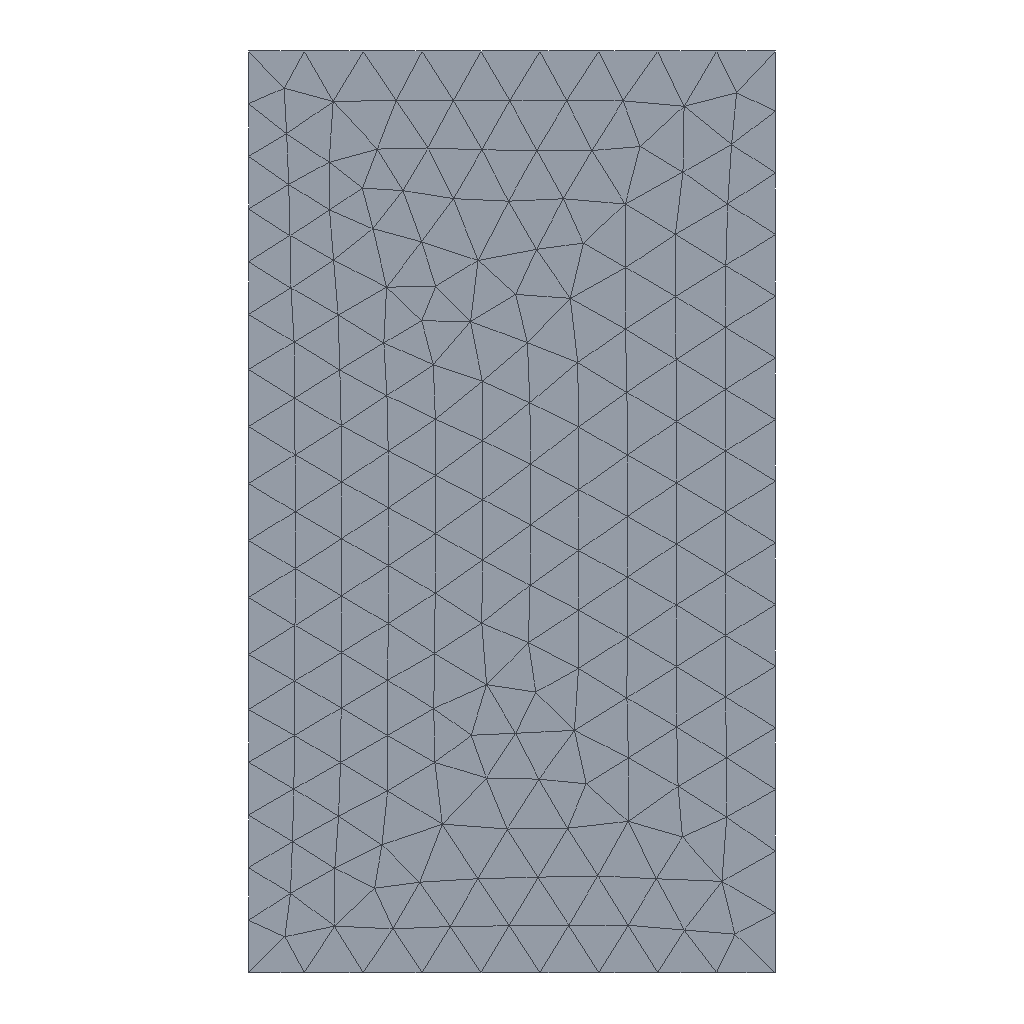Simulation study | comsol
Notes in the study folder:
k_Nb 52.335[W/(m*K)] Thermal conductivity Nb
rho_Nb 8.57e3[kg/m^3] Density Nb
Cp_Nb 2.7e2[J/(kg*K)] Heat capacity Nb
T_0 2.7315e2[K] Boundary temperature
q_0 5e5[W/m^2] Heat flux
Set-up summary:
category,name,step,type,value,unit,region
solver,comsol,,COMSOL Multiphysics 6.4 (Build: 293)
units,SI; geometry length unit m,,stated,COMSOL default unit system (SI)
analysis,Study 1,,Stationary,space_dimension=2D
load_step,std1/stat,std1/stat,Stationary,type=Stationary
mesh,nodes,,,207
mesh,elements,,,362
element_type,tri,,,362
element_type,edg,,,50
element_type,vtx,,,6
component,mod1,,2D,geometry=geom1; domains=1
physics,Heat Transfer (ht),mod1,HeatTransfer,"T(T), discontinuousdamagedtissueindicator(discontinuousdamagedtissueindicator), continuousdamagedtissueindicator(continuousdamagedtissueindicator), thermaldamageindicator(thermaldamageindicator), radiativeintensity(radiativeintensity), incidentradiation(incidentradiation), surfaceradiosity(surfaceradiosity)"
parameter,k_Nb,,,52.335[W/(m*K)]
parameter,rho_Nb,,,8.57e3[kg/m^3]
parameter,Cp_Nb,,,2.7e2[J/(kg*K)]
parameter,T_0,,,2.7315e2[K]
parameter,q_0,,,5e5[W/m^2]
bc,Heat Transfer in Solids 1 (solid1),mod1/ht,SolidHeatTransferModel,k=k_Nb; rho=rho_Nb; Cp=Cp_Nb; streamline=0; crosswind=0; pref=1[atm]; hasPhaseChange=0; Solid_material=dommat; u_prime=0 0 0; dfltopaque=1; thermalConductivityModel=Standard,,selection [1]
bc,Axial Symmetry 1 (axi1),mod1/ht,AxialSymmetry,,,selection []
bc,Thermal Insulation 1 (ins1),mod1/ht,ThermalInsulation,,,"selection [1, 4]"
bc,Initial Values 1 (init1),mod1/ht,init,Tinit=293.15[K]; Tinit_resistive=293.15[K],,selection [1]
bc,Continuity (dcont1),mod1/ht,Continuity,pairDisconnect=1; pairSelection=all; pairsList=0,,selection []
bc,Temperature 1 (temp1),mod1/ht,TemperatureBoundary,T0=T_0,,"selection [2, 5, 6]"
bc,Heat Flux 1 (hf1),mod1/ht,HeatFluxBoundary,HeatFluxType=GeneralInwardHeatFlux; q0_input=q_0; h=0; Text=293.15[K]; P0=0; HeatTransferCoefficientType=UserDef; ExtNaturalConvectionType=VerticalWall; IntNaturalConvectionType=NarrowChimneyParallelPlates; ExtForcedConvectionType=PlateAveragedTransferCoefficient; IntForcedConvectionType=IsothermalTube; ExternalFluidType=Air; Lwall=0; Ldia=0; phi_tilt=0; Ldis=0; Hchimn=0; D=0; Dcyl=0; Dsph=0; Dvcy,,selection [3]
bc,Local Thermal Nonequilibrium Boundary 1 (ltneb1),mod1/ht,LocalThermalNonequilibriumBoundary,,,selection []
COMSOL model file for Java, long lists of numbers shortened:
/*
 * em_deck.java
 */

import com.comsol.model.*;
import com.comsol.model.util.*;

/** Model exported on Oct 28 2026, 10:34 by COMSOL 6.4.0.293. */
public class em_deck {

  public static Model run() {
    Model model = ModelUtil.create("Model");

    model.modelPath("");

    model.label("in.mph");

    model.param().set("k_Nb", "52.335[W/(m*K)]", "Thermal conductivity Nb");
    model.param().set("rho_Nb", "8.57e3[kg/m^3]", "Density Nb");
    model.param().set("Cp_Nb", "2.7e2[J/(kg*K)]", "Heat capacity Nb");
    model.param().set("T_0", "2.7315e2[K]", "Boundary temperature");
    model.param().set("q_0", "5e5[W/m^2]", "Heat flux");

    model.component().create("mod1", false);

    model.component("mod1").geom().create("geom1", 2);

    model.component("mod1").label("Model 1");

    model.component("mod1").defineLocalCoord(false);

    model.component("mod1").curvedInterior(false);

    model.component("mod1").geom("geom1").axisymmetric(true);

    model.component("mod1").mesh().create("mesh1");

    model.component("mod1").geom("geom1").repairTolType("relative");
    model.component("mod1").geom("geom1").create("r1", "Rectangle");
    model.component("mod1").geom("geom1").feature("r1").set("size", new String[]{"8e-2", "1.4e-1"});
    model.component("mod1").geom("geom1").feature("r1").set("pos", new String[]{"2e-2", "0"});
    model.component("mod1").geom("geom1").create("pt1", "Point");
    model.component("mod1").geom("geom1").feature("pt1").set("p", new String[]{"2e-2", "4e-2"});
    model.component("mod1").geom("geom1").create("pt2", "Point");
    model.component("mod1").geom("geom1").feature("pt2").set("p", new String[]{"2e-2", "1e-1"});
    model.component("mod1").geom("geom1").feature("fin").set("repairtoltype", "relative");
    model.component("mod1").geom("geom1").run();

    model.component("mod1").physics().create("ht", "HeatTransfer", "geom1");
    model.component("mod1").physics("ht").create("temp1", "TemperatureBoundary", 1);
    model.component("mod1").physics("ht").feature("temp1").selection().set(2, 5, 6);
    model.component("mod1").physics("ht").create("hf1", "HeatFluxBoundary", 1);
    model.component("mod1").physics("ht").feature("hf1").selection().set(3);

    model.component("mod1").mesh("mesh1").create("ftri1", "FreeTri");

    model.thermodynamics().label("Thermodynamics Package");

    model.component("mod1").view("view1").set("showlabels", true);
    model.component("mod1").view("view1").axis().set("xmin", 0.016);
    model.component("mod1").view("view1").axis().set("xmax", 0.104);
    model.component("mod1").view("view1").axis().set("ymin", -0.01646);
    model.component("mod1").view("view1").axis().set("ymax", 0.1565);

    model.component("mod1").physics("ht").label("Heat Transfer");
    model.component("mod1").physics("ht").prop("ShapeProperty").set("boundaryFlux_temperature", false);
    model.component("mod1").physics("ht").prop("PhysicalModelProperty").set("BackCompStateT", 0);
    model.component("mod1").physics("ht").prop("ConsistentStabilization").set("heatCrosswindDiffusion", false);
    model.component("mod1").physics("ht").prop("ConsistentStabilization").set("StreamlineDiffusionOldForm", true);
    model.component("mod1").physics("ht").prop("ParticipatingMediaSettingsProperty").set("PerfIndex", 0.5);
    model.component("mod1").physics("ht").prop("RadiationSettings").set("lambda_r", "(0)/1[um]");
    model.component("mod1").physics("ht").feature("solid1").set("k_mat", "userdef");
    model.component("mod1").physics("ht").feature("solid1")
         .set("k", new String[][]{{"k_Nb"}, {"0"}, {"0"}, {"0"}, {"k_Nb"}, {"0"}, {"0"}, {"0"}, {"k_Nb"}});
    model.component("mod1").physics("ht").feature("solid1").set("rho_mat", "userdef");
    model.component("mod1").physics("ht").feature("solid1").set("rho", "rho_Nb");
    model.component("mod1").physics("ht").feature("solid1").set("Cp_mat", "userdef");
    model.component("mod1").physics("ht").feature("solid1").set("Cp", "Cp_Nb");
    model.component("mod1").physics("ht").feature("solid1").set("minput_temperature_src", "root.mod1.T");
    model.component("mod1").physics("ht").feature("solid1").set("minput_strainreferencetemperature_src", "userdef");
    model.component("mod1").physics("ht").feature("solid1").set("minput_strainreferencetemperature", 0);
    model.component("mod1").physics("ht").feature("solid1").label("Heat Transfer in Solids 1");
    model.component("mod1").physics("ht").feature("dcont1").set("pairDisconnect", true);
    model.component("mod1").physics("ht").feature("dcont1").label("Continuity");
    model.component("mod1").physics("ht").feature("temp1").set("T0", "T_0");
    model.component("mod1").physics("ht").feature("hf1").set("q0_input", "q_0");

    model.component("mod1").mesh("mesh1").feature("ftri1").set("smoothcontrol", true);
    model.component("mod1").mesh("mesh1").feature("ftri1").set("smoothmaxiter", 8);
    model.component("mod1").mesh("mesh1").feature("ftri1").set("smoothmaxdepth", 8);
    model.component("mod1").mesh("mesh1").run();

    model.study().create("std1");
    model.study("std1").create("stat", "Stationary");

    model.sol().create("sol1");
    model.sol("sol1").attach("std1");
    model.sol("sol1").create("st1", "StudyStep");
    model.sol("sol1").create("v1", "Variables");
    model.sol("sol1").create("s1", "Stationary");
    model.sol("sol1").feature("s1").create("fc1", "FullyCoupled");
    model.sol("sol1").feature("s1").create("d1", "Direct");
    model.sol("sol1").feature("s1").feature().remove("fcDef");

    model.result().create("pg1", "PlotGroup2D");
    model.result("pg1").create("surf1", "Surface");
    model.result("pg1").create("con1", "Contour");

    model.study("std1").feature("stat").set("usestol", true);
    model.study("std1").feature("stat").set("stol", "0.001");

    model.sol("sol1").label("Solver 1");
    model.sol("sol1").feature("st1").label("Compile Equations: Stationary");
    model.sol("sol1").feature("v1").label("Dependent Variables 1.1");
    model.sol("sol1").feature("s1").label("Stationary Solver 1.1");
    model.sol("sol1").feature("s1").set("stol", "0.001");
    model.sol("sol1").feature("s1").feature("dDef").label("Direct 2");
    model.sol("sol1").feature("s1").feature("dDef").set("thresh", 0.1);
    model.sol("sol1").feature("s1").feature("dDef").set("ooc", false);
    model.sol("sol1").feature("s1").feature("dDef").set("rhob", 400);
    model.sol("sol1").feature("s1").feature("aDef").label("Advanced 1");
    model.sol("sol1").feature("s1").feature("fc1").label("Fully Coupled 1.1");
    model.sol("sol1").feature("s1").feature("fc1").set("initstep", 0.01);
    model.sol("sol1").feature("s1").feature("fc1").set("minstep", 1.0E-6);
    model.sol("sol1").feature("s1").feature("fc1").set("maxiter", 50);
    model.sol("sol1").feature("s1").feature("fc1").set("termonres", false);
    model.sol("sol1").feature("s1").feature("fc1").set("probesel", "manual");
    model.sol("sol1").feature("s1").feature("d1").label("Direct 1.1");
    model.sol("sol1").feature("s1").feature("d1").set("linsolver", "pardiso");
    model.sol("sol1").feature("s1").feature("d1").set("ooc", false);
    model.sol("sol1").feature("s1").feature("d1").set("pardreorder", "ndmt");
    model.sol("sol1").feature("s1").feature("d1").set("pivotstrategy", false);
    model.sol("sol1").feature("s1").feature("d1").set("rhob", 400);

    model.study("std1").runNoGen();

    model.result().dataset("dset1").label("Solution 1");
    model.result("pg1").set("smooth", "internal");
    model.result("pg1").feature("surf1").set("colortable", "RainbowClassic");
    model.result("pg1").feature("surf1").set("smooth", "internal");
    model.result("pg1").feature("surf1").set("resolution", "normal");
    model.result("pg1").feature("con1").set("levelrounding", false);
    model.result("pg1").feature("con1").set("colortable", "GrayScale");
    model.result("pg1").feature("con1").set("legendtype", "lines");
    model.result("pg1").feature("con1").set("smooth", "internal");
    model.result("pg1").feature("con1").set("resolution", "normal");

    return model;
  }

  public static void main(String[] args) {
    run();
  }

}
Results summary:
result,max T = abs(mod1.T),dset1 (1 solution(s)),,476.889,K